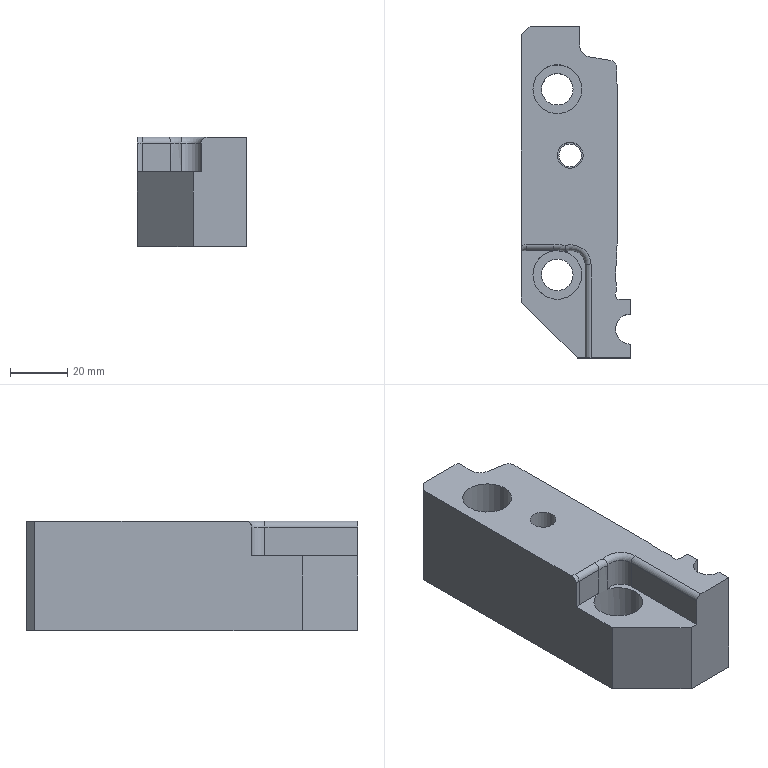Part | STEP file | 1_id106_x_t | 1 solid | 50 faces | box 38 x 115.5 x 38.1 mm | volume 113928 mm3 | plane 22 | cylinder 20 | cone 5 | torus 3 | commonest cylinder face diameters 4 x2 5.4 x2 8.6 x2 10 x2 11 x2 17 x2